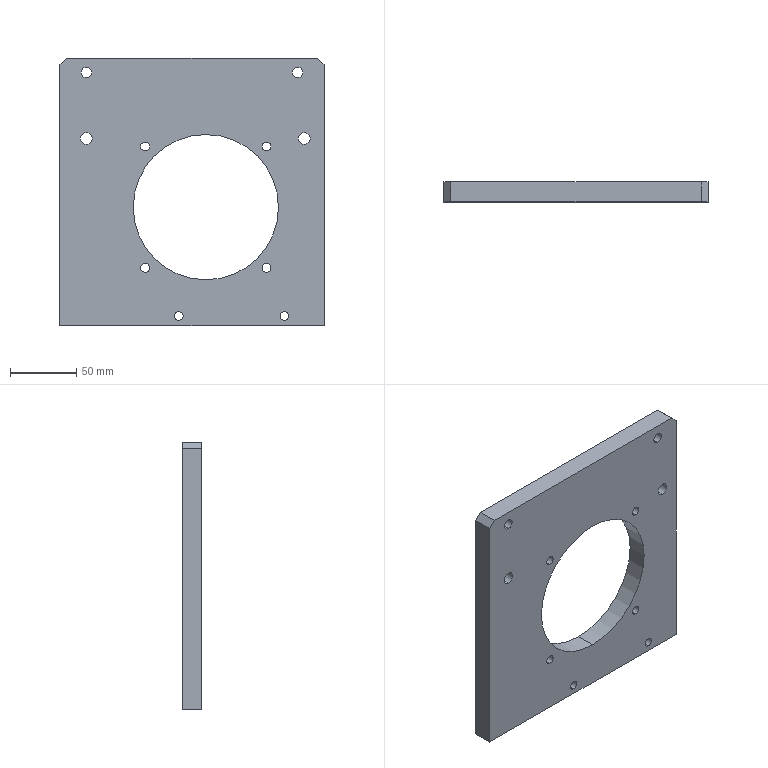Part | STEP file | PN_0011_default | 1 solid | 42 faces | box 200 x 15 x 203 mm | volume 456778 mm3 | cylinder 30 | plane 12 | commonest cylinder face diameters 6.8 x8 6.6 x4 8 x4 9 x4 11 x4 15 x4